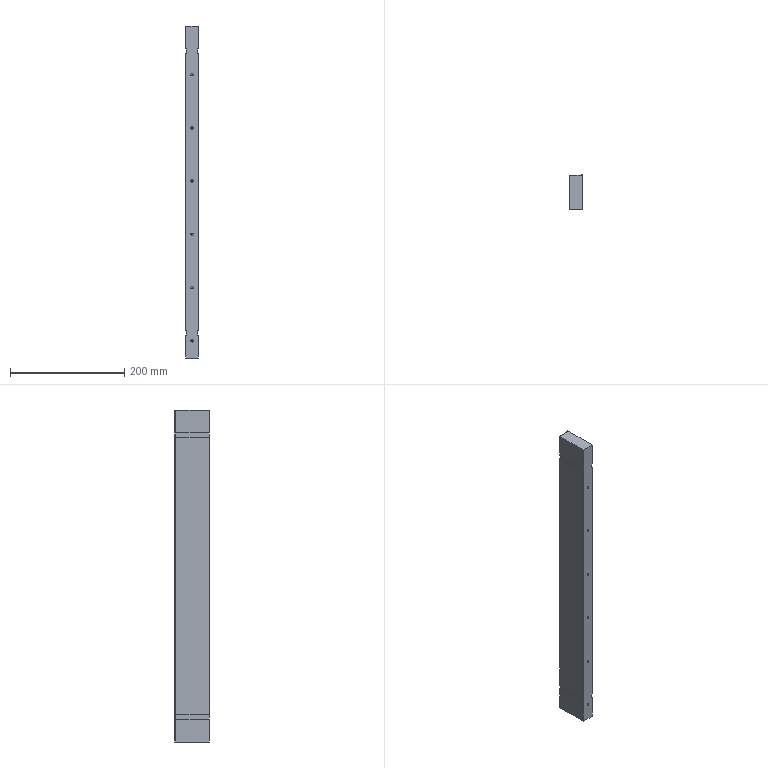Part | NX | features BREP 1 | 1 solid | 88 faces | box 22 x 61 x 580 mm | volume 750398 mm3 | cone 32 | cylinder 32 | plane 24 | commonest cylinder face diameters 4.2 x32